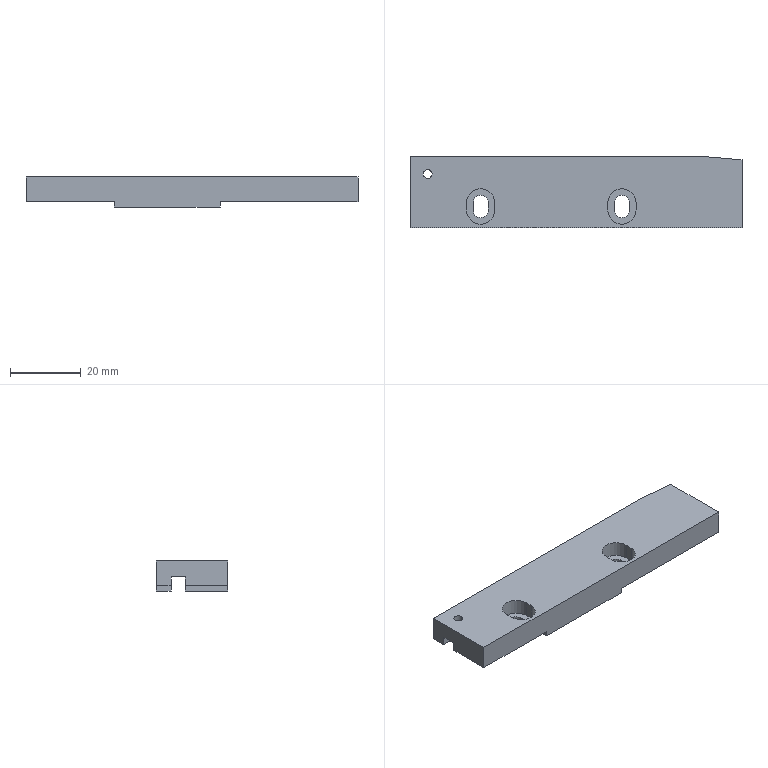Part | NX | features BREP 1 | 1 solid | 40 faces | box 94 x 20.2 x 8.5 mm | volume 12313 mm3 | plane 30 | cylinder 10 | commonest cylinder face diameters 4.3 x4 8 x4 2.5 x2
STEP:
#1=CARTESIAN_POINT('',(-33.75,4.1,2.5));
#2=VERTEX_POINT('',#1);
#3=CARTESIAN_POINT('',(-36.25,4.1,2.5));
#4=VERTEX_POINT('',#3);
#5=CARTESIAN_POINT('',(-35.,4.1,2.5));
#6=DIRECTION('',(0.,0.,-1.));
#7=DIRECTION('',(-1.,0.,0.));
#8=AXIS2_PLACEMENT_3D('',#5,#6,#7);
#9=CIRCLE('',#8,1.25);
#10=EDGE_CURVE('',#2,#4,#9,.T.);
#11=ORIENTED_EDGE('',*,*,#10,.T.);
#12=CARTESIAN_POINT('',(-36.25,4.1,7.));
#13=VERTEX_POINT('',#12);
#14=CARTESIAN_POINT('',(-36.25,4.1,7.));
#15=DIRECTION('',(0.,0.,1.));
#16=VECTOR('',#15,1000.);
#17=LINE('',#14,#16);
#18=EDGE_CURVE('',#13,#4,#17,.F.);
#19=ORIENTED_EDGE('',*,*,#18,.F.);
#20=CARTESIAN_POINT('',(-33.75,4.1,7.));
#21=VERTEX_POINT('',#20);
#22=CARTESIAN_POINT('',(-35.,4.1,7.));
#23=DIRECTION('',(0.,0.,1.));
#24=DIRECTION('',(1.,0.,0.));
#25=AXIS2_PLACEMENT_3D('',#22,#23,#24);
#26=CIRCLE('',#25,1.25);
#27=EDGE_CURVE('',#13,#21,#26,.T.);
#28=ORIENTED_EDGE('',*,*,#27,.T.);
#29=CARTESIAN_POINT('',(-33.75,4.1,7.));
#30=DIRECTION('',(0.,0.,1.));
#31=VECTOR('',#30,1000.);
#32=LINE('',#29,#31);
#33=EDGE_CURVE('',#21,#2,#32,.F.);
#34=ORIENTED_EDGE('',*,*,#33,.T.);
#35=EDGE_LOOP('',(#11,#19,#28,#34));
#36=FACE_BOUND('',#35,.T.);
#37=CARTESIAN_POINT('',(-35.,4.1,7.));
#38=DIRECTION('',(0.,0.,1.));
#39=DIRECTION('',(1.,0.,0.));
#40=AXIS2_PLACEMENT_3D('',#37,#38,#39);
#41=CYLINDRICAL_SURFACE('',#40,1.25);
#42=ADVANCED_FACE('',(#36),#41,.F.);
#43=CARTESIAN_POINT('',(-40.,4.9,0.));
#44=VERTEX_POINT('',#43);
#45=CARTESIAN_POINT('',(-35.96,4.9,0.));
#46=VERTEX_POINT('',#45);
#47=CARTESIAN_POINT('',(0.,4.9,0.));
#48=DIRECTION('',(1.,0.,0.));
#49=VECTOR('',#48,1000.);
#50=LINE('',#47,#49);
#51=EDGE_CURVE('',#44,#46,#50,.T.);
#52=ORIENTED_EDGE('',*,*,#51,.T.);
#53=CARTESIAN_POINT('',(-35.96,4.9,2.5));
#54=VERTEX_POINT('',#53);
#55=CARTESIAN_POINT('',(-35.96,4.9,7.));
#56=DIRECTION('',(0.,0.,1.));
#57=VECTOR('',#56,1000.);
#58=LINE('',#55,#57);
#59=EDGE_CURVE('',#46,#54,#58,.T.);
#60=ORIENTED_EDGE('',*,*,#59,.T.);
#61=CARTESIAN_POINT('',(-40.,4.9,2.5));
#62=VERTEX_POINT('',#61);
#63=CARTESIAN_POINT('',(59.564,4.9,2.5));
#64=DIRECTION('',(1.,0.,0.));
#65=VECTOR('',#64,1000.);
#66=LINE('',#63,#65);
#67=EDGE_CURVE('',#62,#54,#66,.T.);
#68=ORIENTED_EDGE('',*,*,#67,.F.);
#69=CARTESIAN_POINT('',(-40.,4.9,7.));
#70=DIRECTION('',(0.,0.,1.));
#71=VECTOR('',#70,1000.);
#72=LINE('',#69,#71);
#73=EDGE_CURVE('',#44,#62,#72,.T.);
#74=ORIENTED_EDGE('',*,*,#73,.F.);
#75=EDGE_LOOP('',(#52,#60,#68,#74));
#76=FACE_BOUND('',#75,.T.);
#77=CARTESIAN_POINT('',(59.564,4.9,2.5));
#78=DIRECTION('',(0.,1.,0.));
#79=DIRECTION('',(1.,0.,0.));
#80=AXIS2_PLACEMENT_3D('',#77,#78,#79);
#81=PLANE('',#80);
#82=ADVANCED_FACE('',(#76),#81,.F.);
#83=CARTESIAN_POINT('',(54.,0.9,0.));
#84=VERTEX_POINT('',#83);
#85=CARTESIAN_POINT('',(14.98,0.9,0.));
#86=VERTEX_POINT('',#85);
#87=CARTESIAN_POINT('',(0.,0.9,0.));
#88=DIRECTION('',(-1.,0.,0.));
#89=VECTOR('',#88,1000.);
#90=LINE('',#87,#89);
#91=EDGE_CURVE('',#84,#86,#90,.T.);
#92=ORIENTED_EDGE('',*,*,#91,.F.);
#93=CARTESIAN_POINT('',(54.,-11.1,0.));
#94=VERTEX_POINT('',#93);
#95=CARTESIAN_POINT('',(54.,-11.1,0.));
#96=DIRECTION('',(0.,1.,0.));
#97=VECTOR('',#96,1000.);
#98=LINE('',#95,#97);
#99=EDGE_CURVE('',#94,#84,#98,.T.);
#100=ORIENTED_EDGE('',*,*,#99,.F.);
#101=CARTESIAN_POINT('',(14.98,-11.1,0.));
#102=VERTEX_POINT('',#101);
#103=CARTESIAN_POINT('',(-40.,-11.1,0.));
#104=DIRECTION('',(1.,0.,0.));
#105=VECTOR('',#104,1000.);
#106=LINE('',#103,#105);
#107=EDGE_CURVE('',#102,#94,#106,.T.);
#108=ORIENTED_EDGE('',*,*,#107,.F.);
#109=CARTESIAN_POINT('',(14.98,9.1,0.));
#110=DIRECTION('',(0.,-1.,0.));
#111=VECTOR('',#110,1000.);
#112=LINE('',#109,#111);
#113=EDGE_CURVE('',#86,#102,#112,.T.);
#114=ORIENTED_EDGE('',*,*,#113,.F.);
#115=EDGE_LOOP('',(#92,#100,#108,#114));
#116=FACE_BOUND('',#115,.T.);
#117=CARTESIAN_POINT('',(22.15,-4.1,0.));
#118=VERTEX_POINT('',#117);
#119=CARTESIAN_POINT('',(17.85,-4.1,0.));
#120=VERTEX_POINT('',#119);
#121=CARTESIAN_POINT('',(20.,-4.1,0.));
#122=DIRECTION('',(0.,0.,1.));
#123=DIRECTION('',(1.,0.,0.));
#124=AXIS2_PLACEMENT_3D('',#121,#122,#123);
#125=CIRCLE('',#124,2.15);
#126=EDGE_CURVE('',#118,#120,#125,.T.);
#127=ORIENTED_EDGE('',*,*,#126,.T.);
#128=CARTESIAN_POINT('',(17.85,-6.1,0.));
#129=VERTEX_POINT('',#128);
#130=CARTESIAN_POINT('',(17.85,-4.1,0.));
#131=DIRECTION('',(0.,-1.,0.));
#132=VECTOR('',#131,1000.);
#133=LINE('',#130,#132);
#134=EDGE_CURVE('',#120,#129,#133,.T.);
#135=ORIENTED_EDGE('',*,*,#134,.T.);
#136=CARTESIAN_POINT('',(22.15,-6.1,0.));
#137=VERTEX_POINT('',#136);
#138=CARTESIAN_POINT('',(20.,-6.1,0.));
#139=DIRECTION('',(0.,0.,1.));
#140=DIRECTION('',(1.,0.,0.));
#141=AXIS2_PLACEMENT_3D('',#138,#139,#140);
#142=CIRCLE('',#141,2.15);
#143=EDGE_CURVE('',#129,#137,#142,.T.);
#144=ORIENTED_EDGE('',*,*,#143,.T.);
#145=CARTESIAN_POINT('',(22.15,-4.1,0.));
#146=DIRECTION('',(0.,1.,0.));
#147=VECTOR('',#146,1000.);
#148=LINE('',#145,#147);
#149=EDGE_CURVE('',#137,#118,#148,.T.);
#150=ORIENTED_EDGE('',*,*,#149,.T.);
#151=EDGE_LOOP('',(#127,#135,#144,#150));
#152=FACE_BOUND('',#151,.T.);
#153=CARTESIAN_POINT('',(0.,0.,0.));
#154=DIRECTION('',(0.,0.,-1.));
#155=DIRECTION('',(0.,-1.,0.));
#156=AXIS2_PLACEMENT_3D('',#153,#154,#155);
#157=PLANE('',#156);
#158=ADVANCED_FACE('',(#116,#152),#157,.T.);
#159=CARTESIAN_POINT('',(-14.98,0.9,0.));
#160=VERTEX_POINT('',#159);
#161=CARTESIAN_POINT('',(-40.,0.9,0.));
#162=VERTEX_POINT('',#161);
#163=CARTESIAN_POINT('',(0.,0.9,0.));
#164=DIRECTION('',(-1.,0.,0.));
#165=VECTOR('',#164,1000.);
#166=LINE('',#163,#165);
#167=EDGE_CURVE('',#160,#162,#166,.T.);
#168=ORIENTED_EDGE('',*,*,#167,.F.);
#169=CARTESIAN_POINT('',(-14.98,-11.1,0.));
#170=VERTEX_POINT('',#169);
#171=CARTESIAN_POINT('',(-14.98,9.1,0.));
#172=DIRECTION('',(0.,1.,0.));
#173=VECTOR('',#172,1000.);
#174=LINE('',#171,#173);
#175=EDGE_CURVE('',#170,#160,#174,.T.);
#176=ORIENTED_EDGE('',*,*,#175,.F.);
#177=CARTESIAN_POINT('',(-40.,-11.1,0.));
#178=VERTEX_POINT('',#177);
#179=CARTESIAN_POINT('',(-40.,-11.1,0.));
#180=DIRECTION('',(1.,0.,0.));
#181=VECTOR('',#180,1000.);
#182=LINE('',#179,#181);
#183=EDGE_CURVE('',#178,#170,#182,.T.);
#184=ORIENTED_EDGE('',*,*,#183,.F.);
#185=CARTESIAN_POINT('',(-40.,-11.1,0.));
#186=DIRECTION('',(0.,-1.,0.));
#187=VECTOR('',#186,1000.);
#188=LINE('',#185,#187);
#189=EDGE_CURVE('',#162,#178,#188,.T.);
#190=ORIENTED_EDGE('',*,*,#189,.F.);
#191=EDGE_LOOP('',(#168,#176,#184,#190));
#192=FACE_BOUND('',#191,.T.);
#193=CARTESIAN_POINT('',(-17.85,-4.1,0.));
#194=VERTEX_POINT('',#193);
#195=CARTESIAN_POINT('',(-22.15,-4.1,0.));
#196=VERTEX_POINT('',#195);
#197=CARTESIAN_POINT('',(-20.,-4.1,0.));
#198=DIRECTION('',(0.,0.,1.));
#199=DIRECTION('',(1.,0.,0.));
#200=AXIS2_PLACEMENT_3D('',#197,#198,#199);
#201=CIRCLE('',#200,2.15);
#202=EDGE_CURVE('',#194,#196,#201,.T.);
#203=ORIENTED_EDGE('',*,*,#202,.T.);
#204=CARTESIAN_POINT('',(-22.15,-6.1,0.));
#205=VERTEX_POINT('',#204);
#206=CARTESIAN_POINT('',(-22.15,-4.1,0.));
#207=DIRECTION('',(0.,-1.,0.));
#208=VECTOR('',#207,1000.);
#209=LINE('',#206,#208);
#210=EDGE_CURVE('',#196,#205,#209,.T.);
#211=ORIENTED_EDGE('',*,*,#210,.T.);
#212=CARTESIAN_POINT('',(-17.85,-6.1,0.));
#213=VERTEX_POINT('',#212);
#214=CARTESIAN_POINT('',(-20.,-6.1,0.));
#215=DIRECTION('',(0.,0.,1.));
#216=DIRECTION('',(1.,0.,0.));
#217=AXIS2_PLACEMENT_3D('',#214,#215,#216);
#218=CIRCLE('',#217,2.15);
#219=EDGE_CURVE('',#205,#213,#218,.T.);
#220=ORIENTED_EDGE('',*,*,#219,.T.);
#221=CARTESIAN_POINT('',(-17.85,-4.1,0.));
#222=DIRECTION('',(0.,1.,0.));
#223=VECTOR('',#222,1000.);
#224=LINE('',#221,#223);
#225=EDGE_CURVE('',#213,#194,#224,.T.);
#226=ORIENTED_EDGE('',*,*,#225,.T.);
#227=EDGE_LOOP('',(#203,#211,#220,#226));
#228=FACE_BOUND('',#227,.T.);
#229=CARTESIAN_POINT('',(0.,0.,0.));
#230=DIRECTION('',(0.,0.,-1.));
#231=DIRECTION('',(0.,-1.,0.));
#232=AXIS2_PLACEMENT_3D('',#229,#230,#231);
#233=PLANE('',#232);
#234=ADVANCED_FACE('',(#192,#228),#233,.T.);
#235=CARTESIAN_POINT('',(14.98,0.9,-1.5));
#236=VERTEX_POINT('',#235);
#237=CARTESIAN_POINT('',(14.98,-11.1,-1.5));
#238=VERTEX_POINT('',#237);
#239=CARTESIAN_POINT('',(14.98,9.1,-1.5));
#240=DIRECTION('',(0.,-1.,0.));
#241=VECTOR('',#240,1000.);
#242=LINE('',#239,#241);
#243=EDGE_CURVE('',#236,#238,#242,.T.);
#244=ORIENTED_EDGE('',*,*,#243,.F.);
#245=CARTESIAN_POINT('',(14.98,0.9,-1.5));
#246=DIRECTION('',(0.,0.,1.));
#247=VECTOR('',#246,1000.);
#248=LINE('',#245,#247);
#249=EDGE_CURVE('',#236,#86,#248,.T.);
#250=ORIENTED_EDGE('',*,*,#249,.T.);
#251=ORIENTED_EDGE('',*,*,#113,.T.);
#252=CARTESIAN_POINT('',(14.98,-11.1,-1.5));
#253=DIRECTION('',(0.,0.,1.));
#254=VECTOR('',#253,1000.);
#255=LINE('',#252,#254);
#256=EDGE_CURVE('',#238,#102,#255,.T.);
#257=ORIENTED_EDGE('',*,*,#256,.F.);
#258=EDGE_LOOP('',(#244,#250,#251,#257));
#259=FACE_BOUND('',#258,.T.);
#260=CARTESIAN_POINT('',(14.98,9.1,-1.5));
#261=DIRECTION('',(-1.,0.,0.));
#262=DIRECTION('',(0.,0.,1.));
#263=AXIS2_PLACEMENT_3D('',#260,#261,#262);
#264=PLANE('',#263);
#265=ADVANCED_FACE('',(#259),#264,.F.);
#266=ORIENTED_EDGE('',*,*,#175,.T.);
#267=CARTESIAN_POINT('',(-14.98,0.9,-1.5));
#268=VERTEX_POINT('',#267);
#269=CARTESIAN_POINT('',(-14.98,0.9,-1.5));
#270=DIRECTION('',(0.,0.,-1.));
#271=VECTOR('',#270,1000.);
#272=LINE('',#269,#271);
#273=EDGE_CURVE('',#160,#268,#272,.T.);
#274=ORIENTED_EDGE('',*,*,#273,.T.);
#275=CARTESIAN_POINT('',(-14.98,-11.1,-1.5));
#276=VERTEX_POINT('',#275);
#277=CARTESIAN_POINT('',(-14.98,9.1,-1.5));
#278=DIRECTION('',(0.,1.,0.));
#279=VECTOR('',#278,1000.);
#280=LINE('',#277,#279);
#281=EDGE_CURVE('',#276,#268,#280,.T.);
#282=ORIENTED_EDGE('',*,*,#281,.F.);
#283=CARTESIAN_POINT('',(-14.98,-11.1,-1.5));
#284=DIRECTION('',(0.,0.,1.));
#285=VECTOR('',#284,1000.);
#286=LINE('',#283,#285);
#287=EDGE_CURVE('',#276,#170,#286,.T.);
#288=ORIENTED_EDGE('',*,*,#287,.T.);
#289=EDGE_LOOP('',(#266,#274,#282,#288));
#290=FACE_BOUND('',#289,.T.);
#291=CARTESIAN_POINT('',(-14.98,9.1,-1.5));
#292=DIRECTION('',(1.,0.,0.));
#293=DIRECTION('',(0.,-1.,0.));
#294=AXIS2_PLACEMENT_3D('',#291,#292,#293);
#295=PLANE('',#294);
#296=ADVANCED_FACE('',(#290),#295,.F.);
#297=CARTESIAN_POINT('',(0.,0.9,-1.5));
#298=DIRECTION('',(-1.,0.,0.));
#299=VECTOR('',#298,1000.);
#300=LINE('',#297,#299);
#301=EDGE_CURVE('',#236,#268,#300,.T.);
#302=ORIENTED_EDGE('',*,*,#301,.F.);
#303=ORIENTED_EDGE('',*,*,#243,.T.);
#304=CARTESIAN_POINT('',(14.98,-11.1,-1.5));
#305=DIRECTION('',(-1.,0.,0.));
#306=VECTOR('',#305,1000.);
#307=LINE('',#304,#306);
#308=EDGE_CURVE('',#238,#276,#307,.T.);
#309=ORIENTED_EDGE('',*,*,#308,.T.);
#310=ORIENTED_EDGE('',*,*,#281,.T.);
#311=EDGE_LOOP('',(#302,#303,#309,#310));
#312=FACE_BOUND('',#311,.T.);
#313=CARTESIAN_POINT('',(0.,0.,-1.5));
#314=DIRECTION('',(0.,0.,-1.));
#315=DIRECTION('',(0.,-1.,0.));
#316=AXIS2_PLACEMENT_3D('',#313,#314,#315);
#317=PLANE('',#316);
#318=ADVANCED_FACE('',(#312),#317,.T.);
#319=CARTESIAN_POINT('',(14.98,4.9,0.));
#320=VERTEX_POINT('',#319);
#321=CARTESIAN_POINT('',(54.,4.9,0.));
#322=VERTEX_POINT('',#321);
#323=CARTESIAN_POINT('',(0.,4.9,0.));
#324=DIRECTION('',(1.,0.,0.));
#325=VECTOR('',#324,1000.);
#326=LINE('',#323,#325);
#327=EDGE_CURVE('',#320,#322,#326,.T.);
#328=ORIENTED_EDGE('',*,*,#327,.F.);
#329=CARTESIAN_POINT('',(14.98,9.1,0.));
#330=VERTEX_POINT('',#329);
#331=CARTESIAN_POINT('',(14.98,9.1,0.));
#332=DIRECTION('',(0.,-1.,0.));
#333=VECTOR('',#332,1000.);
#334=LINE('',#331,#333);
#335=EDGE_CURVE('',#330,#320,#334,.T.);
#336=ORIENTED_EDGE('',*,*,#335,.F.);
#337=CARTESIAN_POINT('',(42.57,9.1,0.));
#338=VERTEX_POINT('',#337);
#339=CARTESIAN_POINT('',(-40.,9.1,0.));
#340=DIRECTION('',(-1.,0.,0.));
#341=VECTOR('',#340,1000.);
#342=LINE('',#339,#341);
#343=EDGE_CURVE('',#338,#330,#342,.T.);
#344=ORIENTED_EDGE('',*,*,#343,.F.);
#345=CARTESIAN_POINT('',(54.,8.1,0.));
#346=VERTEX_POINT('',#345);
#347=CARTESIAN_POINT('',(15.007,11.511,0.));
#348=DIRECTION('',(0.9962,-0.08716,0.));
#349=VECTOR('',#348,1000.);
#350=LINE('',#347,#349);
#351=EDGE_CURVE('',#338,#346,#350,.T.);
#352=ORIENTED_EDGE('',*,*,#351,.T.);
#353=CARTESIAN_POINT('',(54.,-11.1,0.));
#354=DIRECTION('',(0.,1.,0.));
#355=VECTOR('',#354,1000.);
#356=LINE('',#353,#355);
#357=EDGE_CURVE('',#322,#346,#356,.T.);
#358=ORIENTED_EDGE('',*,*,#357,.F.);
#359=EDGE_LOOP('',(#328,#336,#344,#352,#358));
#360=FACE_BOUND('',#359,.T.);
#361=CARTESIAN_POINT('',(0.,0.,0.));
#362=DIRECTION('',(0.,0.,-1.));
#363=DIRECTION('',(0.,-1.,0.));
#364=AXIS2_PLACEMENT_3D('',#361,#362,#363);
#365=PLANE('',#364);
#366=ADVANCED_FACE('',(#360),#365,.T.);
#367=ORIENTED_EDGE('',*,*,#99,.T.);
#368=CARTESIAN_POINT('',(54.,0.9,2.5));
#369=VERTEX_POINT('',#368);
#370=CARTESIAN_POINT('',(54.,0.9,7.));
#371=DIRECTION('',(0.,0.,1.));
#372=VECTOR('',#371,1000.);
#373=LINE('',#370,#372);
#374=EDGE_CURVE('',#84,#369,#373,.T.);
#375=ORIENTED_EDGE('',*,*,#374,.T.);
#376=CARTESIAN_POINT('',(54.,4.9,2.5));
#377=VERTEX_POINT('',#376);
#378=CARTESIAN_POINT('',(54.,-11.1,2.5));
#379=DIRECTION('',(0.,-1.,0.));
#380=VECTOR('',#379,1000.);
#381=LINE('',#378,#380);
#382=EDGE_CURVE('',#377,#369,#381,.T.);
#383=ORIENTED_EDGE('',*,*,#382,.F.);
#384=CARTESIAN_POINT('',(54.,4.9,7.));
#385=DIRECTION('',(0.,0.,-1.));
#386=VECTOR('',#385,1000.);
#387=LINE('',#384,#386);
#388=EDGE_CURVE('',#377,#322,#387,.T.);
#389=ORIENTED_EDGE('',*,*,#388,.T.);
#390=ORIENTED_EDGE('',*,*,#357,.T.);
#391=CARTESIAN_POINT('',(54.,8.1,7.));
#392=VERTEX_POINT('',#391);
#393=CARTESIAN_POINT('',(54.,8.1,7.));
#394=DIRECTION('',(0.,0.,1.));
#395=VECTOR('',#394,1000.);
#396=LINE('',#393,#395);
#397=EDGE_CURVE('',#346,#392,#396,.T.);
#398=ORIENTED_EDGE('',*,*,#397,.T.);
#399=CARTESIAN_POINT('',(54.,-11.1,7.));
#400=VERTEX_POINT('',#399);
#401=CARTESIAN_POINT('',(54.,-11.1,7.));
#402=DIRECTION('',(0.,1.,0.));
#403=VECTOR('',#402,1000.);
#404=LINE('',#401,#403);
#405=EDGE_CURVE('',#400,#392,#404,.T.);
#406=ORIENTED_EDGE('',*,*,#405,.F.);
#407=CARTESIAN_POINT('',(54.,-11.1,7.));
#408=DIRECTION('',(0.,0.,-1.));
#409=VECTOR('',#408,1000.);
#410=LINE('',#407,#409);
#411=EDGE_CURVE('',#400,#94,#410,.T.);
#412=ORIENTED_EDGE('',*,*,#411,.T.);
#413=EDGE_LOOP('',(#367,#375,#383,#389,#390,#398,#406,#412));
#414=FACE_BOUND('',#413,.T.);
#415=CARTESIAN_POINT('',(54.,-11.1,7.));
#416=DIRECTION('',(-1.,0.,0.));
#417=DIRECTION('',(0.,0.,1.));
#418=AXIS2_PLACEMENT_3D('',#415,#416,#417);
#419=PLANE('',#418);
#420=ADVANCED_FACE('',(#414),#419,.F.);
#421=CARTESIAN_POINT('',(42.57,9.1,7.));
#422=VERTEX_POINT('',#421);
#423=CARTESIAN_POINT('',(-40.,9.1,7.));
#424=VERTEX_POINT('',#423);
#425=CARTESIAN_POINT('',(-40.,9.1,7.));
#426=DIRECTION('',(-1.,0.,0.));
#427=VECTOR('',#426,1000.);
#428=LINE('',#425,#427);
#429=EDGE_CURVE('',#422,#424,#428,.T.);
#430=ORIENTED_EDGE('',*,*,#429,.F.);
#431=CARTESIAN_POINT('',(42.57,9.1,7.));
#432=DIRECTION('',(0.,0.,-1.));
#433=VECTOR('',#432,1000.);
#434=LINE('',#431,#433);
#435=EDGE_CURVE('',#422,#338,#434,.T.);
#436=ORIENTED_EDGE('',*,*,#435,.T.);
#437=ORIENTED_EDGE('',*,*,#343,.T.);
#438=CARTESIAN_POINT('',(14.98,9.1,-1.5));
#439=VERTEX_POINT('',#438);
#440=CARTESIAN_POINT('',(14.98,9.1,-1.5));
#441=DIRECTION('',(0.,0.,1.));
#442=VECTOR('',#441,1000.);
#443=LINE('',#440,#442);
#444=EDGE_CURVE('',#439,#330,#443,.T.);
#445=ORIENTED_EDGE('',*,*,#444,.F.);
#446=CARTESIAN_POINT('',(-14.98,9.1,-1.5));
#447=VERTEX_POINT('',#446);
#448=CARTESIAN_POINT('',(14.98,9.1,-1.5));
#449=DIRECTION('',(1.,0.,0.));
#450=VECTOR('',#449,1000.);
#451=LINE('',#448,#450);
#452=EDGE_CURVE('',#447,#439,#451,.T.);
#453=ORIENTED_EDGE('',*,*,#452,.F.);
#454=CARTESIAN_POINT('',(-14.98,9.1,0.));
#455=VERTEX_POINT('',#454);
#456=CARTESIAN_POINT('',(-14.98,9.1,-1.5));
#457=DIRECTION('',(0.,0.,1.));
#458=VECTOR('',#457,1000.);
#459=LINE('',#456,#458);
#460=EDGE_CURVE('',#447,#455,#459,.T.);
#461=ORIENTED_EDGE('',*,*,#460,.T.);
#462=CARTESIAN_POINT('',(-40.,9.1,0.));
#463=VERTEX_POINT('',#462);
#464=CARTESIAN_POINT('',(-40.,9.1,0.));
#465=DIRECTION('',(-1.,0.,0.));
#466=VECTOR('',#465,1000.);
#467=LINE('',#464,#466);
#468=EDGE_CURVE('',#455,#463,#467,.T.);
#469=ORIENTED_EDGE('',*,*,#468,.T.);
#470=CARTESIAN_POINT('',(-40.,9.1,7.));
#471=DIRECTION('',(0.,0.,-1.));
#472=VECTOR('',#471,1000.);
#473=LINE('',#470,#472);
#474=EDGE_CURVE('',#424,#463,#473,.T.);
#475=ORIENTED_EDGE('',*,*,#474,.F.);
#476=EDGE_LOOP('',(#430,#436,#437,#445,#453,#461,#469,#475));
#477=FACE_BOUND('',#476,.T.);
#478=CARTESIAN_POINT('',(-40.,9.1,7.));
#479=DIRECTION('',(0.,-1.,0.));
#480=DIRECTION('',(0.,0.,-1.));
#481=AXIS2_PLACEMENT_3D('',#478,#479,#480);
#482=PLANE('',#481);
#483=ADVANCED_FACE('',(#477),#482,.F.);
#484=CARTESIAN_POINT('',(-40.,0.9,2.5));
#485=VERTEX_POINT('',#484);
#486=CARTESIAN_POINT('',(-40.,-11.1,2.5));
#487=DIRECTION('',(0.,1.,0.));
#488=VECTOR('',#487,1000.);
#489=LINE('',#486,#488);
#490=EDGE_CURVE('',#485,#62,#489,.T.);
#491=ORIENTED_EDGE('',*,*,#490,.F.);
#492=CARTESIAN_POINT('',(-40.,0.9,7.));
#493=DIRECTION('',(0.,0.,-1.));
#494=VECTOR('',#493,1000.);
#495=LINE('',#492,#494);
#496=EDGE_CURVE('',#485,#162,#495,.T.);
#497=ORIENTED_EDGE('',*,*,#496,.T.);
#498=ORIENTED_EDGE('',*,*,#189,.T.);
#499=CARTESIAN_POINT('',(-40.,-11.1,7.));
#500=VERTEX_POINT('',#499);
#501=CARTESIAN_POINT('',(-40.,-11.1,7.));
#502=DIRECTION('',(0.,0.,-1.));
#503=VECTOR('',#502,1000.);
#504=LINE('',#501,#503);
#505=EDGE_CURVE('',#500,#178,#504,.T.);
#506=ORIENTED_EDGE('',*,*,#505,.F.);
#507=CARTESIAN_POINT('',(-40.,-11.1,7.));
#508=DIRECTION('',(0.,-1.,0.));
#509=VECTOR('',#508,1000.);
#510=LINE('',#507,#509);
#511=EDGE_CURVE('',#424,#500,#510,.T.);
#512=ORIENTED_EDGE('',*,*,#511,.F.);
#513=ORIENTED_EDGE('',*,*,#474,.T.);
#514=CARTESIAN_POINT('',(-40.,-11.1,0.));
#515=DIRECTION('',(0.,-1.,0.));
#516=VECTOR('',#515,1000.);
#517=LINE('',#514,#516);
#518=EDGE_CURVE('',#463,#44,#517,.T.);
#519=ORIENTED_EDGE('',*,*,#518,.T.);
#520=ORIENTED_EDGE('',*,*,#73,.T.);
#521=EDGE_LOOP('',(#491,#497,#498,#506,#512,#513,#519,#520));
#522=FACE_BOUND('',#521,.T.);
#523=CARTESIAN_POINT('',(-40.,-11.1,7.));
#524=DIRECTION('',(1.,0.,0.));
#525=DIRECTION('',(0.,1.,0.));
#526=AXIS2_PLACEMENT_3D('',#523,#524,#525);
#527=PLANE('',#526);
#528=ADVANCED_FACE('',(#522),#527,.F.);
#529=ORIENTED_EDGE('',*,*,#183,.T.);
#530=ORIENTED_EDGE('',*,*,#287,.F.);
#531=ORIENTED_EDGE('',*,*,#308,.F.);
#532=ORIENTED_EDGE('',*,*,#256,.T.);
#533=ORIENTED_EDGE('',*,*,#107,.T.);
#534=ORIENTED_EDGE('',*,*,#411,.F.);
#535=CARTESIAN_POINT('',(-40.,-11.1,7.));
#536=DIRECTION('',(1.,0.,0.));
#537=VECTOR('',#536,1000.);
#538=LINE('',#535,#537);
#539=EDGE_CURVE('',#500,#400,#538,.T.);
#540=ORIENTED_EDGE('',*,*,#539,.F.);
#541=ORIENTED_EDGE('',*,*,#505,.T.);
#542=EDGE_LOOP('',(#529,#530,#531,#532,#533,#534,#540,#541));
#543=FACE_BOUND('',#542,.T.);
#544=CARTESIAN_POINT('',(-40.,-11.1,7.));
#545=DIRECTION('',(0.,1.,0.));
#546=DIRECTION('',(1.,0.,0.));
#547=AXIS2_PLACEMENT_3D('',#544,#545,#546);
#548=PLANE('',#547);
#549=ADVANCED_FACE('',(#543),#548,.F.);
#550=ORIENTED_EDGE('',*,*,#405,.T.);
#551=CARTESIAN_POINT('',(42.57,9.1,7.));
#552=DIRECTION('',(-0.9962,0.08716,0.));
#553=VECTOR('',#552,1000.);
#554=LINE('',#551,#553);
#555=EDGE_CURVE('',#392,#422,#554,.T.);
#556=ORIENTED_EDGE('',*,*,#555,.T.);
#557=ORIENTED_EDGE('',*,*,#429,.T.);
#558=ORIENTED_EDGE('',*,*,#511,.T.);
#559=ORIENTED_EDGE('',*,*,#539,.T.);
#560=EDGE_LOOP('',(#550,#556,#557,#558,#559));
#561=FACE_BOUND('',#560,.T.);
#562=CARTESIAN_POINT('',(-35.,4.1,7.));
#563=DIRECTION('',(0.,0.,1.));
#564=DIRECTION('',(1.,0.,0.));
#565=AXIS2_PLACEMENT_3D('',#562,#563,#564);
#566=CIRCLE('',#565,1.25);
#567=EDGE_CURVE('',#21,#13,#566,.T.);
#568=ORIENTED_EDGE('',*,*,#567,.F.);
#569=ORIENTED_EDGE('',*,*,#27,.F.);
#570=EDGE_LOOP('',(#568,#569));
#571=FACE_BOUND('',#570,.T.);
#572=CARTESIAN_POINT('',(-24.,-4.1,7.));
#573=VERTEX_POINT('',#572);
#574=CARTESIAN_POINT('',(-24.,-6.1,7.));
#575=VERTEX_POINT('',#574);
#576=CARTESIAN_POINT('',(-24.,-6.1,7.));
#577=DIRECTION('',(0.,-1.,0.));
#578=VECTOR('',#577,1000.);
#579=LINE('',#576,#578);
#580=EDGE_CURVE('',#573,#575,#579,.T.);
#581=ORIENTED_EDGE('',*,*,#580,.F.);
#582=CARTESIAN_POINT('',(-16.,-4.1,7.));
#583=VERTEX_POINT('',#582);
#584=CARTESIAN_POINT('',(-20.,-4.1,7.));
#585=DIRECTION('',(0.,0.,1.));
#586=DIRECTION('',(1.,0.,0.));
#587=AXIS2_PLACEMENT_3D('',#584,#585,#586);
#588=CIRCLE('',#587,4.);
#589=EDGE_CURVE('',#583,#573,#588,.T.);
#590=ORIENTED_EDGE('',*,*,#589,.F.);
#591=CARTESIAN_POINT('',(-16.,-6.1,7.));
#592=VERTEX_POINT('',#591);
#593=CARTESIAN_POINT('',(-16.,-6.1,7.));
#594=DIRECTION('',(0.,1.,0.));
#595=VECTOR('',#594,1000.);
#596=LINE('',#593,#595);
#597=EDGE_CURVE('',#592,#583,#596,.T.);
#598=ORIENTED_EDGE('',*,*,#597,.F.);
#599=CARTESIAN_POINT('',(-20.,-6.1,7.));
#600=DIRECTION('',(0.,0.,1.));
#601=DIRECTION('',(1.,0.,0.));
#602=AXIS2_PLACEMENT_3D('',#599,#600,#601);
#603=CIRCLE('',#602,4.);
#604=EDGE_CURVE('',#575,#592,#603,.T.);
#605=ORIENTED_EDGE('',*,*,#604,.F.);
#606=EDGE_LOOP('',(#581,#590,#598,#605));
#607=FACE_BOUND('',#606,.T.);
#608=CARTESIAN_POINT('',(16.,-4.1,7.));
#609=VERTEX_POINT('',#608);
#610=CARTESIAN_POINT('',(16.,-6.1,7.));
#611=VERTEX_POINT('',#610);
#612=CARTESIAN_POINT('',(16.,-6.1,7.));
#613=DIRECTION('',(0.,-1.,0.));
#614=VECTOR('',#613,1000.);
#615=LINE('',#612,#614);
#616=EDGE_CURVE('',#609,#611,#615,.T.);
#617=ORIENTED_EDGE('',*,*,#616,.F.);
#618=CARTESIAN_POINT('',(24.,-4.1,7.));
#619=VERTEX_POINT('',#618);
#620=CARTESIAN_POINT('',(20.,-4.1,7.));
#621=DIRECTION('',(0.,0.,1.));
#622=DIRECTION('',(1.,0.,0.));
#623=AXIS2_PLACEMENT_3D('',#620,#621,#622);
#624=CIRCLE('',#623,4.);
#625=EDGE_CURVE('',#619,#609,#624,.T.);
#626=ORIENTED_EDGE('',*,*,#625,.F.);
#627=CARTESIAN_POINT('',(24.,-6.1,7.));
#628=VERTEX_POINT('',#627);
#629=CARTESIAN_POINT('',(24.,-6.1,7.));
#630=DIRECTION('',(0.,1.,0.));
#631=VECTOR('',#630,1000.);
#632=LINE('',#629,#631);
#633=EDGE_CURVE('',#628,#619,#632,.T.);
#634=ORIENTED_EDGE('',*,*,#633,.F.);
#635=CARTESIAN_POINT('',(20.,-6.1,7.));
#636=DIRECTION('',(0.,0.,1.));
#637=DIRECTION('',(1.,0.,0.));
#638=AXIS2_PLACEMENT_3D('',#635,#636,#637);
#639=CIRCLE('',#638,4.);
#640=EDGE_CURVE('',#611,#628,#639,.T.);
#641=ORIENTED_EDGE('',*,*,#640,.F.);
#642=EDGE_LOOP('',(#617,#626,#634,#641));
#643=FACE_BOUND('',#642,.T.);
#644=CARTESIAN_POINT('',(0.,0.,7.));
#645=DIRECTION('',(0.,0.,-1.));
#646=DIRECTION('',(0.,-1.,0.));
#647=AXIS2_PLACEMENT_3D('',#644,#645,#646);
#648=PLANE('',#647);
#649=ADVANCED_FACE('',(#561,#571,#607,#643),#648,.F.);
#650=CARTESIAN_POINT('',(-34.04,4.9,0.));
#651=VERTEX_POINT('',#650);
#652=CARTESIAN_POINT('',(-35.,4.1,0.));
#653=DIRECTION('',(0.,0.,-1.));
#654=DIRECTION('',(-1.,0.,0.));
#655=AXIS2_PLACEMENT_3D('',#652,#653,#654);
#656=CIRCLE('',#655,1.25);
#657=EDGE_CURVE('',#46,#651,#656,.T.);
#658=ORIENTED_EDGE('',*,*,#657,.F.);
#659=ORIENTED_EDGE('',*,*,#51,.F.);
#660=ORIENTED_EDGE('',*,*,#518,.F.);
#661=ORIENTED_EDGE('',*,*,#468,.F.);
#662=CARTESIAN_POINT('',(-14.98,4.9,0.));
#663=VERTEX_POINT('',#662);
#664=CARTESIAN_POINT('',(-14.98,9.1,0.));
#665=DIRECTION('',(0.,1.,0.));
#666=VECTOR('',#665,1000.);
#667=LINE('',#664,#666);
#668=EDGE_CURVE('',#663,#455,#667,.T.);
#669=ORIENTED_EDGE('',*,*,#668,.F.);
#670=CARTESIAN_POINT('',(0.,4.9,0.));
#671=DIRECTION('',(1.,0.,0.));
#672=VECTOR('',#671,1000.);
#673=LINE('',#670,#672);
#674=EDGE_CURVE('',#651,#663,#673,.T.);
#675=ORIENTED_EDGE('',*,*,#674,.F.);
#676=EDGE_LOOP('',(#658,#659,#660,#661,#669,#675));
#677=FACE_BOUND('',#676,.T.);
#678=CARTESIAN_POINT('',(0.,0.,0.));
#679=DIRECTION('',(0.,0.,-1.));
#680=DIRECTION('',(0.,-1.,0.));
#681=AXIS2_PLACEMENT_3D('',#678,#679,#680);
#682=PLANE('',#681);
#683=ADVANCED_FACE('',(#677),#682,.T.);
#684=CARTESIAN_POINT('',(-16.,-4.1,2.6));
#685=VERTEX_POINT('',#684);
#686=CARTESIAN_POINT('',(-24.,-4.1,2.6));
#687=VERTEX_POINT('',#686);
#688=CARTESIAN_POINT('',(-20.,-4.1,2.6));
#689=DIRECTION('',(0.,0.,1.));
#690=DIRECTION('',(-1.,0.,0.));
#691=AXIS2_PLACEMENT_3D('',#688,#689,#690);
#692=CIRCLE('',#691,4.);
#693=EDGE_CURVE('',#685,#687,#692,.T.);
#694=ORIENTED_EDGE('',*,*,#693,.T.);
#695=CARTESIAN_POINT('',(-24.,-6.1,2.6));
#696=VERTEX_POINT('',#695);
#697=CARTESIAN_POINT('',(-24.,-6.1,2.6));
#698=DIRECTION('',(0.,-1.,0.));
#699=VECTOR('',#698,1000.);
#700=LINE('',#697,#699);
#701=EDGE_CURVE('',#687,#696,#700,.T.);
#702=ORIENTED_EDGE('',*,*,#701,.T.);
#703=CARTESIAN_POINT('',(-16.,-6.1,2.6));
#704=VERTEX_POINT('',#703);
#705=CARTESIAN_POINT('',(-20.,-6.1,2.6));
#706=DIRECTION('',(0.,0.,1.));
#707=DIRECTION('',(-1.,0.,0.));
#708=AXIS2_PLACEMENT_3D('',#705,#706,#707);
#709=CIRCLE('',#708,4.);
#710=EDGE_CURVE('',#696,#704,#709,.T.);
#711=ORIENTED_EDGE('',*,*,#710,.T.);
#712=CARTESIAN_POINT('',(-16.,-6.1,2.6));
#713=DIRECTION('',(0.,1.,0.));
#714=VECTOR('',#713,1000.);
#715=LINE('',#712,#714);
#716=EDGE_CURVE('',#704,#685,#715,.T.);
#717=ORIENTED_EDGE('',*,*,#716,.T.);
#718=EDGE_LOOP('',(#694,#702,#711,#717));
#719=FACE_BOUND('',#718,.T.);
#720=CARTESIAN_POINT('',(-22.15,-6.1,2.6));
#721=VERTEX_POINT('',#720);
#722=CARTESIAN_POINT('',(-22.15,-4.1,2.6));
#723=VERTEX_POINT('',#722);
#724=CARTESIAN_POINT('',(-22.15,-5.1,2.6));
#725=DIRECTION('',(0.,1.,0.));
#726=VECTOR('',#725,1000.);
#727=LINE('',#724,#726);
#728=EDGE_CURVE('',#721,#723,#727,.T.);
#729=ORIENTED_EDGE('',*,*,#728,.T.);
#730=CARTESIAN_POINT('',(-17.85,-4.1,2.6));
#731=VERTEX_POINT('',#730);
#732=CARTESIAN_POINT('',(-20.,-4.1,2.6));
#733=DIRECTION('',(0.,0.,1.));
#734=DIRECTION('',(1.,0.,0.));
#735=AXIS2_PLACEMENT_3D('',#732,#733,#734);
#736=CIRCLE('',#735,2.15);
#737=EDGE_CURVE('',#731,#723,#736,.T.);
#738=ORIENTED_EDGE('',*,*,#737,.F.);
#739=CARTESIAN_POINT('',(-17.85,-6.1,2.6));
#740=VERTEX_POINT('',#739);
#741=CARTESIAN_POINT('',(-17.85,-5.1,2.6));
#742=DIRECTION('',(0.,-1.,0.));
#743=VECTOR('',#742,1000.);
#744=LINE('',#741,#743);
#745=EDGE_CURVE('',#731,#740,#744,.T.);
#746=ORIENTED_EDGE('',*,*,#745,.T.);
#747=CARTESIAN_POINT('',(-20.,-6.1,2.6));
#748=DIRECTION('',(0.,0.,1.));
#749=DIRECTION('',(1.,0.,0.));
#750=AXIS2_PLACEMENT_3D('',#747,#748,#749);
#751=CIRCLE('',#750,2.15);
#752=EDGE_CURVE('',#721,#740,#751,.T.);
#753=ORIENTED_EDGE('',*,*,#752,.F.);
#754=EDGE_LOOP('',(#729,#738,#746,#753));
#755=FACE_BOUND('',#754,.T.);
#756=CARTESIAN_POINT('',(-17.85,-5.1,2.6));
#757=DIRECTION('',(0.,0.,-1.));
#758=DIRECTION('',(0.,-1.,0.));
#759=AXIS2_PLACEMENT_3D('',#756,#757,#758);
#760=PLANE('',#759);
#761=ADVANCED_FACE('',(#719,#755),#760,.F.);
#762=CARTESIAN_POINT('',(24.,-4.1,2.6));
#763=VERTEX_POINT('',#762);
#764=CARTESIAN_POINT('',(16.,-4.1,2.6));
#765=VERTEX_POINT('',#764);
#766=CARTESIAN_POINT('',(20.,-4.1,2.6));
#767=DIRECTION('',(0.,0.,1.));
#768=DIRECTION('',(-1.,0.,0.));
#769=AXIS2_PLACEMENT_3D('',#766,#767,#768);
#770=CIRCLE('',#769,4.);
#771=EDGE_CURVE('',#763,#765,#770,.T.);
#772=ORIENTED_EDGE('',*,*,#771,.T.);
#773=CARTESIAN_POINT('',(16.,-6.1,2.6));
#774=VERTEX_POINT('',#773);
#775=CARTESIAN_POINT('',(16.,-6.1,2.6));
#776=DIRECTION('',(0.,-1.,0.));
#777=VECTOR('',#776,1000.);
#778=LINE('',#775,#777);
#779=EDGE_CURVE('',#765,#774,#778,.T.);
#780=ORIENTED_EDGE('',*,*,#779,.T.);
#781=CARTESIAN_POINT('',(24.,-6.1,2.6));
#782=VERTEX_POINT('',#781);
#783=CARTESIAN_POINT('',(20.,-6.1,2.6));
#784=DIRECTION('',(0.,0.,1.));
#785=DIRECTION('',(-1.,0.,0.));
#786=AXIS2_PLACEMENT_3D('',#783,#784,#785);
#787=CIRCLE('',#786,4.);
#788=EDGE_CURVE('',#774,#782,#787,.T.);
#789=ORIENTED_EDGE('',*,*,#788,.T.);
#790=CARTESIAN_POINT('',(24.,-6.1,2.6));
#791=DIRECTION('',(0.,1.,0.));
#792=VECTOR('',#791,1000.);
#793=LINE('',#790,#792);
#794=EDGE_CURVE('',#782,#763,#793,.T.);
#795=ORIENTED_EDGE('',*,*,#794,.T.);
#796=EDGE_LOOP('',(#772,#780,#789,#795));
#797=FACE_BOUND('',#796,.T.);
#798=CARTESIAN_POINT('',(17.85,-6.1,2.6));
#799=VERTEX_POINT('',#798);
#800=CARTESIAN_POINT('',(17.85,-4.1,2.6));
#801=VERTEX_POINT('',#800);
#802=CARTESIAN_POINT('',(17.85,-5.1,2.6));
#803=DIRECTION('',(0.,1.,0.));
#804=VECTOR('',#803,1000.);
#805=LINE('',#802,#804);
#806=EDGE_CURVE('',#799,#801,#805,.T.);
#807=ORIENTED_EDGE('',*,*,#806,.T.);
#808=CARTESIAN_POINT('',(22.15,-4.1,2.6));
#809=VERTEX_POINT('',#808);
#810=CARTESIAN_POINT('',(20.,-4.1,2.6));
#811=DIRECTION('',(0.,0.,1.));
#812=DIRECTION('',(1.,0.,0.));
#813=AXIS2_PLACEMENT_3D('',#810,#811,#812);
#814=CIRCLE('',#813,2.15);
#815=EDGE_CURVE('',#809,#801,#814,.T.);
#816=ORIENTED_EDGE('',*,*,#815,.F.);
#817=CARTESIAN_POINT('',(22.15,-6.1,2.6));
#818=VERTEX_POINT('',#817);
#819=CARTESIAN_POINT('',(22.15,-5.1,2.6));
#820=DIRECTION('',(0.,-1.,0.));
#821=VECTOR('',#820,1000.);
#822=LINE('',#819,#821);
#823=EDGE_CURVE('',#809,#818,#822,.T.);
#824=ORIENTED_EDGE('',*,*,#823,.T.);
#825=CARTESIAN_POINT('',(20.,-6.1,2.6));
#826=DIRECTION('',(0.,0.,1.));
#827=DIRECTION('',(1.,0.,0.));
#828=AXIS2_PLACEMENT_3D('',#825,#826,#827);
#829=CIRCLE('',#828,2.15);
#830=EDGE_CURVE('',#799,#818,#829,.T.);
#831=ORIENTED_EDGE('',*,*,#830,.F.);
#832=EDGE_LOOP('',(#807,#816,#824,#831));
#833=FACE_BOUND('',#832,.T.);
#834=CARTESIAN_POINT('',(22.15,-5.1,2.6));
#835=DIRECTION('',(0.,0.,-1.));
#836=DIRECTION('',(0.,-1.,0.));
#837=AXIS2_PLACEMENT_3D('',#834,#835,#836);
#838=PLANE('',#837);
#839=ADVANCED_FACE('',(#797,#833),#838,.F.);
#840=ORIENTED_EDGE('',*,*,#555,.F.);
#841=ORIENTED_EDGE('',*,*,#397,.F.);
#842=ORIENTED_EDGE('',*,*,#351,.F.);
#843=ORIENTED_EDGE('',*,*,#435,.F.);
#844=EDGE_LOOP('',(#840,#841,#842,#843));
#845=FACE_BOUND('',#844,.T.);
#846=CARTESIAN_POINT('',(42.57,9.1,7.));
#847=DIRECTION('',(-0.08716,-0.9962,0.));
#848=DIRECTION('',(-0.9962,0.08716,0.));
#849=AXIS2_PLACEMENT_3D('',#846,#847,#848);
#850=PLANE('',#849);
#851=ADVANCED_FACE('',(#845),#850,.F.);
#852=ORIENTED_EDGE('',*,*,#633,.T.);
#853=CARTESIAN_POINT('',(24.,-4.1,-10.206));
#854=DIRECTION('',(0.,0.,1.));
#855=VECTOR('',#854,1000.);
#856=LINE('',#853,#855);
#857=EDGE_CURVE('',#763,#619,#856,.T.);
#858=ORIENTED_EDGE('',*,*,#857,.F.);
#859=ORIENTED_EDGE('',*,*,#794,.F.);
#860=CARTESIAN_POINT('',(24.,-6.1,-10.206));
#861=DIRECTION('',(0.,0.,1.));
#862=VECTOR('',#861,1000.);
#863=LINE('',#860,#862);
#864=EDGE_CURVE('',#782,#628,#863,.T.);
#865=ORIENTED_EDGE('',*,*,#864,.T.);
#866=EDGE_LOOP('',(#852,#858,#859,#865));
#867=FACE_BOUND('',#866,.T.);
#868=CARTESIAN_POINT('',(24.,-6.1,-10.206));
#869=DIRECTION('',(1.,0.,0.));
#870=DIRECTION('',(0.,1.,0.));
#871=AXIS2_PLACEMENT_3D('',#868,#869,#870);
#872=PLANE('',#871);
#873=ADVANCED_FACE('',(#867),#872,.F.);
#874=ORIENTED_EDGE('',*,*,#616,.T.);
#875=CARTESIAN_POINT('',(16.,-6.1,-10.206));
#876=DIRECTION('',(0.,0.,1.));
#877=VECTOR('',#876,1000.);
#878=LINE('',#875,#877);
#879=EDGE_CURVE('',#774,#611,#878,.T.);
#880=ORIENTED_EDGE('',*,*,#879,.F.);
#881=ORIENTED_EDGE('',*,*,#779,.F.);
#882=CARTESIAN_POINT('',(16.,-4.1,-10.206));
#883=DIRECTION('',(0.,0.,1.));
#884=VECTOR('',#883,1000.);
#885=LINE('',#882,#884);
#886=EDGE_CURVE('',#765,#609,#885,.T.);
#887=ORIENTED_EDGE('',*,*,#886,.T.);
#888=EDGE_LOOP('',(#874,#880,#881,#887));
#889=FACE_BOUND('',#888,.T.);
#890=CARTESIAN_POINT('',(16.,-6.1,-10.206));
#891=DIRECTION('',(-1.,0.,0.));
#892=DIRECTION('',(0.,0.,1.));
#893=AXIS2_PLACEMENT_3D('',#890,#891,#892);
#894=PLANE('',#893);
#895=ADVANCED_FACE('',(#889),#894,.F.);
#896=ORIENTED_EDGE('',*,*,#857,.T.);
#897=ORIENTED_EDGE('',*,*,#625,.T.);
#898=ORIENTED_EDGE('',*,*,#886,.F.);
#899=ORIENTED_EDGE('',*,*,#771,.F.);
#900=EDGE_LOOP('',(#896,#897,#898,#899));
#901=FACE_BOUND('',#900,.T.);
#902=CARTESIAN_POINT('',(20.,-4.1,-10.206));
#903=DIRECTION('',(0.,0.,1.));
#904=DIRECTION('',(1.,0.,0.));
#905=AXIS2_PLACEMENT_3D('',#902,#903,#904);
#906=CYLINDRICAL_SURFACE('',#905,4.);
#907=ADVANCED_FACE('',(#901),#906,.F.);
#908=ORIENTED_EDGE('',*,*,#879,.T.);
#909=ORIENTED_EDGE('',*,*,#640,.T.);
#910=ORIENTED_EDGE('',*,*,#864,.F.);
#911=ORIENTED_EDGE('',*,*,#788,.F.);
#912=EDGE_LOOP('',(#908,#909,#910,#911));
#913=FACE_BOUND('',#912,.T.);
#914=CARTESIAN_POINT('',(20.,-6.1,-10.206));
#915=DIRECTION('',(0.,0.,1.));
#916=DIRECTION('',(1.,0.,0.));
#917=AXIS2_PLACEMENT_3D('',#914,#915,#916);
#918=CYLINDRICAL_SURFACE('',#917,4.);
#919=ADVANCED_FACE('',(#913),#918,.F.);
#920=ORIENTED_EDGE('',*,*,#823,.F.);
#921=CARTESIAN_POINT('',(22.15,-4.1,0.));
#922=DIRECTION('',(0.,0.,1.));
#923=VECTOR('',#922,1000.);
#924=LINE('',#921,#923);
#925=EDGE_CURVE('',#118,#809,#924,.T.);
#926=ORIENTED_EDGE('',*,*,#925,.F.);
#927=ORIENTED_EDGE('',*,*,#149,.F.);
#928=CARTESIAN_POINT('',(22.15,-6.1,0.));
#929=DIRECTION('',(0.,0.,1.));
#930=VECTOR('',#929,1000.);
#931=LINE('',#928,#930);
#932=EDGE_CURVE('',#137,#818,#931,.T.);
#933=ORIENTED_EDGE('',*,*,#932,.T.);
#934=EDGE_LOOP('',(#920,#926,#927,#933));
#935=FACE_BOUND('',#934,.T.);
#936=CARTESIAN_POINT('',(22.15,-4.1,0.));
#937=DIRECTION('',(1.,0.,0.));
#938=DIRECTION('',(0.,1.,0.));
#939=AXIS2_PLACEMENT_3D('',#936,#937,#938);
#940=PLANE('',#939);
#941=ADVANCED_FACE('',(#935),#940,.F.);
#942=ORIENTED_EDGE('',*,*,#806,.F.);
#943=CARTESIAN_POINT('',(17.85,-6.1,0.));
#944=DIRECTION('',(0.,0.,1.));
#945=VECTOR('',#944,1000.);
#946=LINE('',#943,#945);
#947=EDGE_CURVE('',#129,#799,#946,.T.);
#948=ORIENTED_EDGE('',*,*,#947,.F.);
#949=ORIENTED_EDGE('',*,*,#134,.F.);
#950=CARTESIAN_POINT('',(17.85,-4.1,0.));
#951=DIRECTION('',(0.,0.,1.));
#952=VECTOR('',#951,1000.);
#953=LINE('',#950,#952);
#954=EDGE_CURVE('',#120,#801,#953,.T.);
#955=ORIENTED_EDGE('',*,*,#954,.T.);
#956=EDGE_LOOP('',(#942,#948,#949,#955));
#957=FACE_BOUND('',#956,.T.);
#958=CARTESIAN_POINT('',(17.85,-4.1,0.));
#959=DIRECTION('',(-1.,0.,0.));
#960=DIRECTION('',(0.,0.,1.));
#961=AXIS2_PLACEMENT_3D('',#958,#959,#960);
#962=PLANE('',#961);
#963=ADVANCED_FACE('',(#957),#962,.F.);
#964=ORIENTED_EDGE('',*,*,#815,.T.);
#965=ORIENTED_EDGE('',*,*,#954,.F.);
#966=ORIENTED_EDGE('',*,*,#126,.F.);
#967=ORIENTED_EDGE('',*,*,#925,.T.);
#968=EDGE_LOOP('',(#964,#965,#966,#967));
#969=FACE_BOUND('',#968,.T.);
#970=CARTESIAN_POINT('',(20.,-4.1,0.));
#971=DIRECTION('',(0.,0.,1.));
#972=DIRECTION('',(1.,0.,0.));
#973=AXIS2_PLACEMENT_3D('',#970,#971,#972);
#974=CYLINDRICAL_SURFACE('',#973,2.15);
#975=ADVANCED_FACE('',(#969),#974,.F.);
#976=ORIENTED_EDGE('',*,*,#830,.T.);
#977=ORIENTED_EDGE('',*,*,#932,.F.);
#978=ORIENTED_EDGE('',*,*,#143,.F.);
#979=ORIENTED_EDGE('',*,*,#947,.T.);
#980=EDGE_LOOP('',(#976,#977,#978,#979));
#981=FACE_BOUND('',#980,.T.);
#982=CARTESIAN_POINT('',(20.,-6.1,0.));
#983=DIRECTION('',(0.,0.,1.));
#984=DIRECTION('',(1.,0.,0.));
#985=AXIS2_PLACEMENT_3D('',#982,#983,#984);
#986=CYLINDRICAL_SURFACE('',#985,2.15);
#987=ADVANCED_FACE('',(#981),#986,.F.);
#988=ORIENTED_EDGE('',*,*,#597,.T.);
#989=CARTESIAN_POINT('',(-16.,-4.1,-10.206));
#990=DIRECTION('',(0.,0.,1.));
#991=VECTOR('',#990,1000.);
#992=LINE('',#989,#991);
#993=EDGE_CURVE('',#685,#583,#992,.T.);
#994=ORIENTED_EDGE('',*,*,#993,.F.);
#995=ORIENTED_EDGE('',*,*,#716,.F.);
#996=CARTESIAN_POINT('',(-16.,-6.1,-10.206));
#997=DIRECTION('',(0.,0.,1.));
#998=VECTOR('',#997,1000.);
#999=LINE('',#996,#998);
#1000=EDGE_CURVE('',#704,#592,#999,.T.);
#1001=ORIENTED_EDGE('',*,*,#1000,.T.);
#1002=EDGE_LOOP('',(#988,#994,#995,#1001));
#1003=FACE_BOUND('',#1002,.T.);
#1004=CARTESIAN_POINT('',(-16.,-6.1,-10.206));
#1005=DIRECTION('',(1.,0.,0.));
#1006=DIRECTION('',(0.,1.,0.));
#1007=AXIS2_PLACEMENT_3D('',#1004,#1005,#1006);
#1008=PLANE('',#1007);
#1009=ADVANCED_FACE('',(#1003),#1008,.F.);
#1010=ORIENTED_EDGE('',*,*,#580,.T.);
#1011=CARTESIAN_POINT('',(-24.,-6.1,-10.206));
#1012=DIRECTION('',(0.,0.,1.));
#1013=VECTOR('',#1012,1000.);
#1014=LINE('',#1011,#1013);
#1015=EDGE_CURVE('',#696,#575,#1014,.T.);
#1016=ORIENTED_EDGE('',*,*,#1015,.F.);
#1017=ORIENTED_EDGE('',*,*,#701,.F.);
#1018=CARTESIAN_POINT('',(-24.,-4.1,-10.206));
#1019=DIRECTION('',(0.,0.,1.));
#1020=VECTOR('',#1019,1000.);
#1021=LINE('',#1018,#1020);
#1022=EDGE_CURVE('',#687,#573,#1021,.T.);
#1023=ORIENTED_EDGE('',*,*,#1022,.T.);
#1024=EDGE_LOOP('',(#1010,#1016,#1017,#1023));
#1025=FACE_BOUND('',#1024,.T.);
#1026=CARTESIAN_POINT('',(-24.,-6.1,-10.206));
#1027=DIRECTION('',(-1.,0.,0.));
#1028=DIRECTION('',(0.,0.,1.));
#1029=AXIS2_PLACEMENT_3D('',#1026,#1027,#1028);
#1030=PLANE('',#1029);
#1031=ADVANCED_FACE('',(#1025),#1030,.F.);
#1032=ORIENTED_EDGE('',*,*,#993,.T.);
#1033=ORIENTED_EDGE('',*,*,#589,.T.);
#1034=ORIENTED_EDGE('',*,*,#1022,.F.);
#1035=ORIENTED_EDGE('',*,*,#693,.F.);
#1036=EDGE_LOOP('',(#1032,#1033,#1034,#1035));
#1037=FACE_BOUND('',#1036,.T.);
#1038=CARTESIAN_POINT('',(-20.,-4.1,-10.206));
#1039=DIRECTION('',(0.,0.,1.));
#1040=DIRECTION('',(1.,0.,0.));
#1041=AXIS2_PLACEMENT_3D('',#1038,#1039,#1040);
#1042=CYLINDRICAL_SURFACE('',#1041,4.);
#1043=ADVANCED_FACE('',(#1037),#1042,.F.);
#1044=ORIENTED_EDGE('',*,*,#1015,.T.);
#1045=ORIENTED_EDGE('',*,*,#604,.T.);
#1046=ORIENTED_EDGE('',*,*,#1000,.F.);
#1047=ORIENTED_EDGE('',*,*,#710,.F.);
#1048=EDGE_LOOP('',(#1044,#1045,#1046,#1047));
#1049=FACE_BOUND('',#1048,.T.);
#1050=CARTESIAN_POINT('',(-20.,-6.1,-10.206));
#1051=DIRECTION('',(0.,0.,1.));
#1052=DIRECTION('',(1.,0.,0.));
#1053=AXIS2_PLACEMENT_3D('',#1050,#1051,#1052);
#1054=CYLINDRICAL_SURFACE('',#1053,4.);
#1055=ADVANCED_FACE('',(#1049),#1054,.F.);
#1056=ORIENTED_EDGE('',*,*,#745,.F.);
#1057=CARTESIAN_POINT('',(-17.85,-4.1,0.));
#1058=DIRECTION('',(0.,0.,1.));
#1059=VECTOR('',#1058,1000.);
#1060=LINE('',#1057,#1059);
#1061=EDGE_CURVE('',#194,#731,#1060,.T.);
#1062=ORIENTED_EDGE('',*,*,#1061,.F.);
#1063=ORIENTED_EDGE('',*,*,#225,.F.);
#1064=CARTESIAN_POINT('',(-17.85,-6.1,0.));
#1065=DIRECTION('',(0.,0.,1.));
#1066=VECTOR('',#1065,1000.);
#1067=LINE('',#1064,#1066);
#1068=EDGE_CURVE('',#213,#740,#1067,.T.);
#1069=ORIENTED_EDGE('',*,*,#1068,.T.);
#1070=EDGE_LOOP('',(#1056,#1062,#1063,#1069));
#1071=FACE_BOUND('',#1070,.T.);
#1072=CARTESIAN_POINT('',(-17.85,-4.1,0.));
#1073=DIRECTION('',(1.,0.,0.));
#1074=DIRECTION('',(0.,1.,0.));
#1075=AXIS2_PLACEMENT_3D('',#1072,#1073,#1074);
#1076=PLANE('',#1075);
#1077=ADVANCED_FACE('',(#1071),#1076,.F.);
#1078=ORIENTED_EDGE('',*,*,#728,.F.);
#1079=CARTESIAN_POINT('',(-22.15,-6.1,0.));
#1080=DIRECTION('',(0.,0.,1.));
#1081=VECTOR('',#1080,1000.);
#1082=LINE('',#1079,#1081);
#1083=EDGE_CURVE('',#205,#721,#1082,.T.);
#1084=ORIENTED_EDGE('',*,*,#1083,.F.);
#1085=ORIENTED_EDGE('',*,*,#210,.F.);
#1086=CARTESIAN_POINT('',(-22.15,-4.1,0.));
#1087=DIRECTION('',(0.,0.,1.));
#1088=VECTOR('',#1087,1000.);
#1089=LINE('',#1086,#1088);
#1090=EDGE_CURVE('',#196,#723,#1089,.T.);
#1091=ORIENTED_EDGE('',*,*,#1090,.T.);
#1092=EDGE_LOOP('',(#1078,#1084,#1085,#1091));
#1093=FACE_BOUND('',#1092,.T.);
#1094=CARTESIAN_POINT('',(-22.15,-4.1,0.));
#1095=DIRECTION('',(-1.,0.,0.));
#1096=DIRECTION('',(0.,0.,1.));
#1097=AXIS2_PLACEMENT_3D('',#1094,#1095,#1096);
#1098=PLANE('',#1097);
#1099=ADVANCED_FACE('',(#1093),#1098,.F.);
#1100=ORIENTED_EDGE('',*,*,#737,.T.);
#1101=ORIENTED_EDGE('',*,*,#1090,.F.);
#1102=ORIENTED_EDGE('',*,*,#202,.F.);
#1103=ORIENTED_EDGE('',*,*,#1061,.T.);
#1104=EDGE_LOOP('',(#1100,#1101,#1102,#1103));
#1105=FACE_BOUND('',#1104,.T.);
#1106=CARTESIAN_POINT('',(-20.,-4.1,0.));
#1107=DIRECTION('',(0.,0.,1.));
#1108=DIRECTION('',(1.,0.,0.));
#1109=AXIS2_PLACEMENT_3D('',#1106,#1107,#1108);
#1110=CYLINDRICAL_SURFACE('',#1109,2.15);
#1111=ADVANCED_FACE('',(#1105),#1110,.F.);
#1112=ORIENTED_EDGE('',*,*,#752,.T.);
#1113=ORIENTED_EDGE('',*,*,#1068,.F.);
#1114=ORIENTED_EDGE('',*,*,#219,.F.);
#1115=ORIENTED_EDGE('',*,*,#1083,.T.);
#1116=EDGE_LOOP('',(#1112,#1113,#1114,#1115));
#1117=FACE_BOUND('',#1116,.T.);
#1118=CARTESIAN_POINT('',(-20.,-6.1,0.));
#1119=DIRECTION('',(0.,0.,1.));
#1120=DIRECTION('',(1.,0.,0.));
#1121=AXIS2_PLACEMENT_3D('',#1118,#1119,#1120);
#1122=CYLINDRICAL_SURFACE('',#1121,2.15);
#1123=ADVANCED_FACE('',(#1117),#1122,.F.);
#1124=ORIENTED_EDGE('',*,*,#335,.T.);
#1125=CARTESIAN_POINT('',(14.98,4.9,-1.5));
#1126=VERTEX_POINT('',#1125);
#1127=CARTESIAN_POINT('',(14.98,4.9,-1.5));
#1128=DIRECTION('',(0.,0.,-1.));
#1129=VECTOR('',#1128,1000.);
#1130=LINE('',#1127,#1129);
#1131=EDGE_CURVE('',#320,#1126,#1130,.T.);
#1132=ORIENTED_EDGE('',*,*,#1131,.T.);
#1133=CARTESIAN_POINT('',(14.98,9.1,-1.5));
#1134=DIRECTION('',(0.,-1.,0.));
#1135=VECTOR('',#1134,1000.);
#1136=LINE('',#1133,#1135);
#1137=EDGE_CURVE('',#439,#1126,#1136,.T.);
#1138=ORIENTED_EDGE('',*,*,#1137,.F.);
#1139=ORIENTED_EDGE('',*,*,#444,.T.);
#1140=EDGE_LOOP('',(#1124,#1132,#1138,#1139));
#1141=FACE_BOUND('',#1140,.T.);
#1142=CARTESIAN_POINT('',(14.98,9.1,-1.5));
#1143=DIRECTION('',(-1.,0.,0.));
#1144=DIRECTION('',(0.,0.,1.));
#1145=AXIS2_PLACEMENT_3D('',#1142,#1143,#1144);
#1146=PLANE('',#1145);
#1147=ADVANCED_FACE('',(#1141),#1146,.F.);
#1148=CARTESIAN_POINT('',(-14.98,4.9,-1.5));
#1149=VERTEX_POINT('',#1148);
#1150=CARTESIAN_POINT('',(-14.98,9.1,-1.5));
#1151=DIRECTION('',(0.,1.,0.));
#1152=VECTOR('',#1151,1000.);
#1153=LINE('',#1150,#1152);
#1154=EDGE_CURVE('',#1149,#447,#1153,.T.);
#1155=ORIENTED_EDGE('',*,*,#1154,.F.);
#1156=CARTESIAN_POINT('',(-14.98,4.9,-1.5));
#1157=DIRECTION('',(0.,0.,1.));
#1158=VECTOR('',#1157,1000.);
#1159=LINE('',#1156,#1158);
#1160=EDGE_CURVE('',#1149,#663,#1159,.T.);
#1161=ORIENTED_EDGE('',*,*,#1160,.T.);
#1162=ORIENTED_EDGE('',*,*,#668,.T.);
#1163=ORIENTED_EDGE('',*,*,#460,.F.);
#1164=EDGE_LOOP('',(#1155,#1161,#1162,#1163));
#1165=FACE_BOUND('',#1164,.T.);
#1166=CARTESIAN_POINT('',(-14.98,9.1,-1.5));
#1167=DIRECTION('',(1.,0.,0.));
#1168=DIRECTION('',(0.,-1.,0.));
#1169=AXIS2_PLACEMENT_3D('',#1166,#1167,#1168);
#1170=PLANE('',#1169);
#1171=ADVANCED_FACE('',(#1165),#1170,.F.);
#1172=CARTESIAN_POINT('',(0.,4.9,-1.5));
#1173=DIRECTION('',(1.,0.,0.));
#1174=VECTOR('',#1173,1000.);
#1175=LINE('',#1172,#1174);
#1176=EDGE_CURVE('',#1149,#1126,#1175,.T.);
#1177=ORIENTED_EDGE('',*,*,#1176,.F.);
#1178=ORIENTED_EDGE('',*,*,#1154,.T.);
#1179=ORIENTED_EDGE('',*,*,#452,.T.);
#1180=ORIENTED_EDGE('',*,*,#1137,.T.);
#1181=EDGE_LOOP('',(#1177,#1178,#1179,#1180));
#1182=FACE_BOUND('',#1181,.T.);
#1183=CARTESIAN_POINT('',(0.,0.,-1.5));
#1184=DIRECTION('',(0.,0.,-1.));
#1185=DIRECTION('',(0.,-1.,0.));
#1186=AXIS2_PLACEMENT_3D('',#1183,#1184,#1185);
#1187=PLANE('',#1186);
#1188=ADVANCED_FACE('',(#1182),#1187,.T.);
#1189=CARTESIAN_POINT('',(-34.04,4.9,2.5));
#1190=VERTEX_POINT('',#1189);
#1191=CARTESIAN_POINT('',(-35.,4.1,2.5));
#1192=DIRECTION('',(0.,0.,-1.));
#1193=DIRECTION('',(-1.,0.,0.));
#1194=AXIS2_PLACEMENT_3D('',#1191,#1192,#1193);
#1195=CIRCLE('',#1194,1.25);
#1196=EDGE_CURVE('',#1190,#2,#1195,.T.);
#1197=ORIENTED_EDGE('',*,*,#1196,.F.);
#1198=CARTESIAN_POINT('',(59.564,4.9,2.5));
#1199=DIRECTION('',(1.,0.,0.));
#1200=VECTOR('',#1199,1000.);
#1201=LINE('',#1198,#1200);
#1202=EDGE_CURVE('',#1190,#377,#1201,.T.);
#1203=ORIENTED_EDGE('',*,*,#1202,.T.);
#1204=ORIENTED_EDGE('',*,*,#382,.T.);
#1205=CARTESIAN_POINT('',(59.564,0.9,2.5));
#1206=DIRECTION('',(-1.,0.,0.));
#1207=VECTOR('',#1206,1000.);
#1208=LINE('',#1205,#1207);
#1209=EDGE_CURVE('',#369,#485,#1208,.T.);
#1210=ORIENTED_EDGE('',*,*,#1209,.T.);
#1211=ORIENTED_EDGE('',*,*,#490,.T.);
#1212=ORIENTED_EDGE('',*,*,#67,.T.);
#1213=CARTESIAN_POINT('',(-35.,4.1,2.5));
#1214=DIRECTION('',(0.,0.,-1.));
#1215=DIRECTION('',(-1.,0.,0.));
#1216=AXIS2_PLACEMENT_3D('',#1213,#1214,#1215);
#1217=CIRCLE('',#1216,1.25);
#1218=EDGE_CURVE('',#4,#54,#1217,.T.);
#1219=ORIENTED_EDGE('',*,*,#1218,.F.);
#1220=ORIENTED_EDGE('',*,*,#10,.F.);
#1221=EDGE_LOOP('',(#1197,#1203,#1204,#1210,#1211,#1212,#1219,#1220));
#1222=FACE_BOUND('',#1221,.T.);
#1223=CARTESIAN_POINT('',(0.,0.,2.5));
#1224=DIRECTION('',(0.,0.,-1.));
#1225=DIRECTION('',(0.,-1.,0.));
#1226=AXIS2_PLACEMENT_3D('',#1223,#1224,#1225);
#1227=PLANE('',#1226);
#1228=ADVANCED_FACE('',(#1222),#1227,.T.);
#1229=ORIENTED_EDGE('',*,*,#91,.T.);
#1230=ORIENTED_EDGE('',*,*,#249,.F.);
#1231=ORIENTED_EDGE('',*,*,#301,.T.);
#1232=ORIENTED_EDGE('',*,*,#273,.F.);
#1233=ORIENTED_EDGE('',*,*,#167,.T.);
#1234=ORIENTED_EDGE('',*,*,#496,.F.);
#1235=ORIENTED_EDGE('',*,*,#1209,.F.);
#1236=ORIENTED_EDGE('',*,*,#374,.F.);
#1237=EDGE_LOOP('',(#1229,#1230,#1231,#1232,#1233,#1234,#1235,#1236));
#1238=FACE_BOUND('',#1237,.T.);
#1239=CARTESIAN_POINT('',(59.564,0.9,2.5));
#1240=DIRECTION('',(0.,-1.,0.));
#1241=DIRECTION('',(0.,0.,-1.));
#1242=AXIS2_PLACEMENT_3D('',#1239,#1240,#1241);
#1243=PLANE('',#1242);
#1244=ADVANCED_FACE('',(#1238),#1243,.F.);
#1245=ORIENTED_EDGE('',*,*,#1202,.F.);
#1246=CARTESIAN_POINT('',(-34.04,4.9,7.));
#1247=DIRECTION('',(0.,0.,-1.));
#1248=VECTOR('',#1247,1000.);
#1249=LINE('',#1246,#1248);
#1250=EDGE_CURVE('',#1190,#651,#1249,.T.);
#1251=ORIENTED_EDGE('',*,*,#1250,.T.);
#1252=ORIENTED_EDGE('',*,*,#674,.T.);
#1253=ORIENTED_EDGE('',*,*,#1160,.F.);
#1254=ORIENTED_EDGE('',*,*,#1176,.T.);
#1255=ORIENTED_EDGE('',*,*,#1131,.F.);
#1256=ORIENTED_EDGE('',*,*,#327,.T.);
#1257=ORIENTED_EDGE('',*,*,#388,.F.);
#1258=EDGE_LOOP('',(#1245,#1251,#1252,#1253,#1254,#1255,#1256,#1257));
#1259=FACE_BOUND('',#1258,.T.);
#1260=CARTESIAN_POINT('',(59.564,4.9,2.5));
#1261=DIRECTION('',(0.,1.,0.));
#1262=DIRECTION('',(1.,0.,0.));
#1263=AXIS2_PLACEMENT_3D('',#1260,#1261,#1262);
#1264=PLANE('',#1263);
#1265=ADVANCED_FACE('',(#1259),#1264,.F.);
#1266=ORIENTED_EDGE('',*,*,#18,.T.);
#1267=ORIENTED_EDGE('',*,*,#1218,.T.);
#1268=ORIENTED_EDGE('',*,*,#59,.F.);
#1269=ORIENTED_EDGE('',*,*,#657,.T.);
#1270=ORIENTED_EDGE('',*,*,#1250,.F.);
#1271=ORIENTED_EDGE('',*,*,#1196,.T.);
#1272=ORIENTED_EDGE('',*,*,#33,.F.);
#1273=ORIENTED_EDGE('',*,*,#567,.T.);
#1274=EDGE_LOOP('',(#1266,#1267,#1268,#1269,#1270,#1271,#1272,#1273));
#1275=FACE_BOUND('',#1274,.T.);
#1276=CARTESIAN_POINT('',(-35.,4.1,7.));
#1277=DIRECTION('',(0.,0.,1.));
#1278=DIRECTION('',(1.,0.,0.));
#1279=AXIS2_PLACEMENT_3D('',#1276,#1277,#1278);
#1280=CYLINDRICAL_SURFACE('',#1279,1.25);
#1281=ADVANCED_FACE('',(#1275),#1280,.F.);
#1282=CLOSED_SHELL('',(#42,#82,#158,#234,#265,#296,#318,#366,#420,#483,#528,#549,#649,#683,#761,#839,#851,#873,#895,#907,#919,#941,#963,#975,#987,#1009,#1031,#1043,#1055,#1077,#1099,#1111,#1123,#1147,#1171,#1188,#1228,#1244,#1265,#1281));
#1283=MANIFOLD_SOLID_BREP('',#1282);
#1284=(LENGTH_UNIT()NAMED_UNIT(*)SI_UNIT(.MILLI.,.METRE.));
#1285=UNCERTAINTY_MEASURE_WITH_UNIT(LENGTH_MEASURE(0.00001),#1284,'','');
#1286=(NAMED_UNIT(*)PLANE_ANGLE_UNIT()SI_UNIT($,.RADIAN.));
#1287=(NAMED_UNIT(*)SI_UNIT($,.STERADIAN.)SOLID_ANGLE_UNIT());
#1288=(GEOMETRIC_REPRESENTATION_CONTEXT(3)GLOBAL_UNCERTAINTY_ASSIGNED_CONTEXT((#1285))GLOBAL_UNIT_ASSIGNED_CONTEXT((#1284,#1286,#1287))REPRESENTATION_CONTEXT('',''));
#1289=ADVANCED_BREP_SHAPE_REPRESENTATION('',(#1283),#1288);